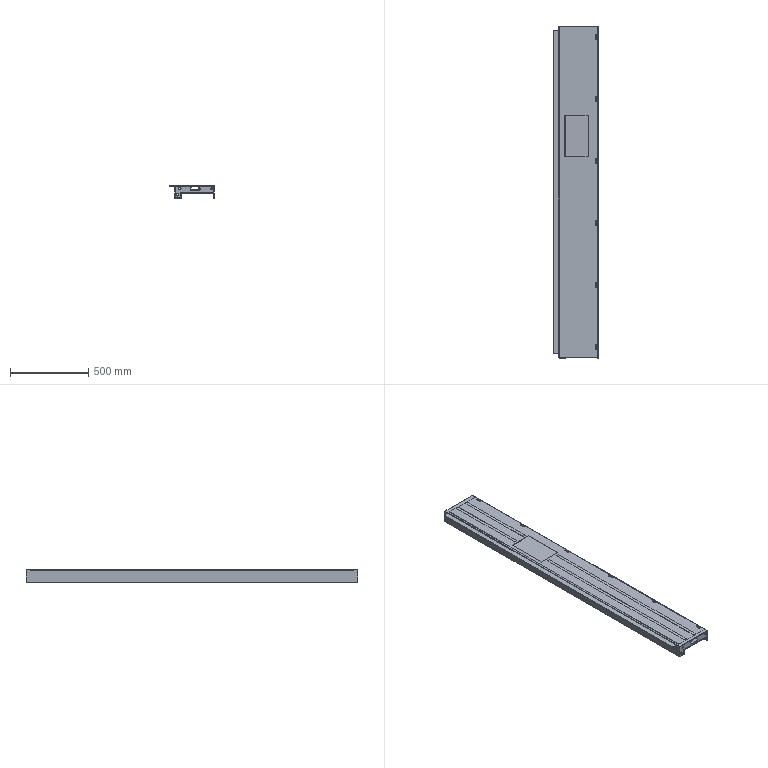Part | SolidWorks | 9 solids | 618 faces | box 282.3 x 2116 x 80 mm | volume 2341732 mm3 | plane 370 | cylinder 248 | commonest cylinder face diameters 6 x116 6.2 x28 9 x18 2 x15 6.1 x10 11 x10